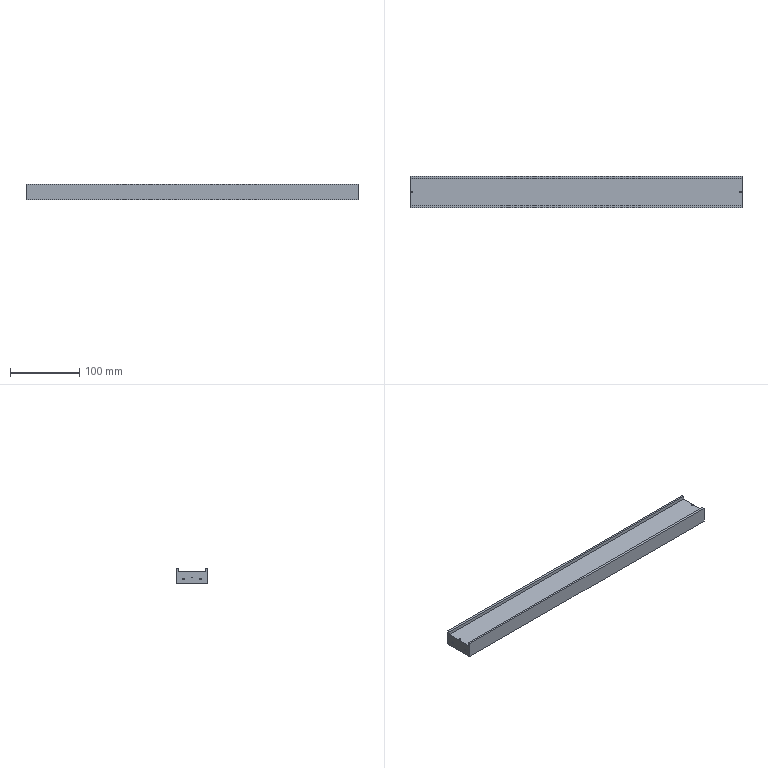Part | NX | 1 solid | 27 faces | box 480 x 45 x 23 mm | volume 314022 mm3 | plane 15 | cone 6 | cylinder 6 | commonest cylinder face diameters 2.5 x6
STEP:
#1=CARTESIAN_POINT('',(240.,-22.5,23.));
#2=VERTEX_POINT('',#1);
#3=CARTESIAN_POINT('',(240.,-19.5,23.));
#4=VERTEX_POINT('',#3);
#5=CARTESIAN_POINT('',(240.,-22.5,23.));
#6=DIRECTION('',(0.,1.,0.));
#7=VECTOR('',#6,1000.);
#8=LINE('',#5,#7);
#9=EDGE_CURVE('',#2,#4,#8,.T.);
#10=ORIENTED_EDGE('',*,*,#9,.T.);
#11=CARTESIAN_POINT('',(-240.,-19.5,23.));
#12=VERTEX_POINT('',#11);
#13=CARTESIAN_POINT('',(-240.,-19.5,23.));
#14=DIRECTION('',(1.,0.,0.));
#15=VECTOR('',#14,1000.);
#16=LINE('',#13,#15);
#17=EDGE_CURVE('',#12,#4,#16,.T.);
#18=ORIENTED_EDGE('',*,*,#17,.F.);
#19=CARTESIAN_POINT('',(-240.,-22.5,23.));
#20=VERTEX_POINT('',#19);
#21=CARTESIAN_POINT('',(-240.,-22.5,23.));
#22=DIRECTION('',(0.,-1.,0.));
#23=VECTOR('',#22,1000.);
#24=LINE('',#21,#23);
#25=EDGE_CURVE('',#12,#20,#24,.T.);
#26=ORIENTED_EDGE('',*,*,#25,.T.);
#27=CARTESIAN_POINT('',(-240.,-22.5,23.));
#28=DIRECTION('',(1.,0.,0.));
#29=VECTOR('',#28,1000.);
#30=LINE('',#27,#29);
#31=EDGE_CURVE('',#20,#2,#30,.T.);
#32=ORIENTED_EDGE('',*,*,#31,.T.);
#33=EDGE_LOOP('',(#10,#18,#26,#32));
#34=FACE_BOUND('',#33,.T.);
#35=CARTESIAN_POINT('',(0.,0.,23.));
#36=DIRECTION('',(0.,0.,-1.));
#37=DIRECTION('',(-1.,0.,0.));
#38=AXIS2_PLACEMENT_3D('',#35,#36,#37);
#39=PLANE('',#38);
#40=ADVANCED_FACE('',(#34),#39,.F.);
#41=CARTESIAN_POINT('',(240.,12.5,5.75));
#42=VERTEX_POINT('',#41);
#43=CARTESIAN_POINT('',(240.,12.5,7.));
#44=DIRECTION('',(1.,0.,0.));
#45=DIRECTION('',(0.,0.,-1.));
#46=AXIS2_PLACEMENT_3D('',#43,#44,#45);
#47=CIRCLE('',#46,1.25);
#48=EDGE_CURVE('',#42,#42,#47,.T.);
#49=ORIENTED_EDGE('',*,*,#48,.F.);
#50=EDGE_LOOP('',(#49));
#51=FACE_BOUND('',#50,.T.);
#52=CARTESIAN_POINT('',(240.,-12.5,5.75));
#53=VERTEX_POINT('',#52);
#54=CARTESIAN_POINT('',(240.,-12.5,7.));
#55=DIRECTION('',(1.,0.,0.));
#56=DIRECTION('',(0.,0.,-1.));
#57=AXIS2_PLACEMENT_3D('',#54,#55,#56);
#58=CIRCLE('',#57,1.25);
#59=EDGE_CURVE('',#53,#53,#58,.T.);
#60=ORIENTED_EDGE('',*,*,#59,.F.);
#61=EDGE_LOOP('',(#60));
#62=FACE_BOUND('',#61,.T.);
#63=CARTESIAN_POINT('',(240.,-19.5,18.));
#64=VERTEX_POINT('',#63);
#65=CARTESIAN_POINT('',(240.,19.5,18.));
#66=VERTEX_POINT('',#65);
#67=CARTESIAN_POINT('',(240.,-19.5,18.));
#68=DIRECTION('',(0.,1.,0.));
#69=VECTOR('',#68,1000.);
#70=LINE('',#67,#69);
#71=EDGE_CURVE('',#64,#66,#70,.T.);
#72=ORIENTED_EDGE('',*,*,#71,.F.);
#73=CARTESIAN_POINT('',(240.,-19.5,18.));
#74=DIRECTION('',(0.,0.,1.));
#75=VECTOR('',#74,1000.);
#76=LINE('',#73,#75);
#77=EDGE_CURVE('',#64,#4,#76,.T.);
#78=ORIENTED_EDGE('',*,*,#77,.T.);
#79=ORIENTED_EDGE('',*,*,#9,.F.);
#80=CARTESIAN_POINT('',(240.,-22.5,0.));
#81=VERTEX_POINT('',#80);
#82=CARTESIAN_POINT('',(240.,-22.5,23.));
#83=DIRECTION('',(0.,0.,-1.));
#84=VECTOR('',#83,1000.);
#85=LINE('',#82,#84);
#86=EDGE_CURVE('',#2,#81,#85,.T.);
#87=ORIENTED_EDGE('',*,*,#86,.T.);
#88=CARTESIAN_POINT('',(240.,22.5,0.));
#89=VERTEX_POINT('',#88);
#90=CARTESIAN_POINT('',(240.,-22.5,0.));
#91=DIRECTION('',(0.,1.,0.));
#92=VECTOR('',#91,1000.);
#93=LINE('',#90,#92);
#94=EDGE_CURVE('',#81,#89,#93,.T.);
#95=ORIENTED_EDGE('',*,*,#94,.T.);
#96=CARTESIAN_POINT('',(240.,22.5,23.));
#97=VERTEX_POINT('',#96);
#98=CARTESIAN_POINT('',(240.,22.5,23.));
#99=DIRECTION('',(0.,0.,-1.));
#100=VECTOR('',#99,1000.);
#101=LINE('',#98,#100);
#102=EDGE_CURVE('',#97,#89,#101,.T.);
#103=ORIENTED_EDGE('',*,*,#102,.F.);
#104=CARTESIAN_POINT('',(240.,19.5,23.));
#105=VERTEX_POINT('',#104);
#106=CARTESIAN_POINT('',(240.,-22.5,23.));
#107=DIRECTION('',(0.,1.,0.));
#108=VECTOR('',#107,1000.);
#109=LINE('',#106,#108);
#110=EDGE_CURVE('',#105,#97,#109,.T.);
#111=ORIENTED_EDGE('',*,*,#110,.F.);
#112=CARTESIAN_POINT('',(240.,19.5,18.));
#113=DIRECTION('',(0.,0.,1.));
#114=VECTOR('',#113,1000.);
#115=LINE('',#112,#114);
#116=EDGE_CURVE('',#66,#105,#115,.T.);
#117=ORIENTED_EDGE('',*,*,#116,.F.);
#118=EDGE_LOOP('',(#72,#78,#79,#87,#95,#103,#111,#117));
#119=FACE_BOUND('',#118,.T.);
#120=CARTESIAN_POINT('',(240.,-22.5,23.));
#121=DIRECTION('',(-1.,0.,0.));
#122=DIRECTION('',(0.,0.,1.));
#123=AXIS2_PLACEMENT_3D('',#120,#121,#122);
#124=PLANE('',#123);
#125=ADVANCED_FACE('',(#51,#62,#119),#124,.F.);
#126=CARTESIAN_POINT('',(-240.,22.5,0.));
#127=VERTEX_POINT('',#126);
#128=CARTESIAN_POINT('',(-240.,22.5,0.));
#129=DIRECTION('',(-1.,0.,0.));
#130=VECTOR('',#129,1000.);
#131=LINE('',#128,#130);
#132=EDGE_CURVE('',#89,#127,#131,.T.);
#133=ORIENTED_EDGE('',*,*,#132,.T.);
#134=CARTESIAN_POINT('',(-240.,22.5,23.));
#135=VERTEX_POINT('',#134);
#136=CARTESIAN_POINT('',(-240.,22.5,23.));
#137=DIRECTION('',(0.,0.,-1.));
#138=VECTOR('',#137,1000.);
#139=LINE('',#136,#138);
#140=EDGE_CURVE('',#135,#127,#139,.T.);
#141=ORIENTED_EDGE('',*,*,#140,.F.);
#142=CARTESIAN_POINT('',(-240.,22.5,23.));
#143=DIRECTION('',(-1.,0.,0.));
#144=VECTOR('',#143,1000.);
#145=LINE('',#142,#144);
#146=EDGE_CURVE('',#97,#135,#145,.T.);
#147=ORIENTED_EDGE('',*,*,#146,.F.);
#148=ORIENTED_EDGE('',*,*,#102,.T.);
#149=EDGE_LOOP('',(#133,#141,#147,#148));
#150=FACE_BOUND('',#149,.T.);
#151=CARTESIAN_POINT('',(-240.,22.5,23.));
#152=DIRECTION('',(0.,-1.,0.));
#153=DIRECTION('',(0.,0.,-1.));
#154=AXIS2_PLACEMENT_3D('',#151,#152,#153);
#155=PLANE('',#154);
#156=ADVANCED_FACE('',(#150),#155,.F.);
#157=CARTESIAN_POINT('',(-240.,12.5,8.25));
#158=VERTEX_POINT('',#157);
#159=CARTESIAN_POINT('',(-240.,12.5,7.));
#160=DIRECTION('',(-1.,0.,0.));
#161=DIRECTION('',(0.,0.,1.));
#162=AXIS2_PLACEMENT_3D('',#159,#160,#161);
#163=CIRCLE('',#162,1.25);
#164=EDGE_CURVE('',#158,#158,#163,.T.);
#165=ORIENTED_EDGE('',*,*,#164,.F.);
#166=EDGE_LOOP('',(#165));
#167=FACE_BOUND('',#166,.T.);
#168=CARTESIAN_POINT('',(-240.,-12.5,8.25));
#169=VERTEX_POINT('',#168);
#170=CARTESIAN_POINT('',(-240.,-12.5,7.));
#171=DIRECTION('',(-1.,0.,0.));
#172=DIRECTION('',(0.,0.,1.));
#173=AXIS2_PLACEMENT_3D('',#170,#171,#172);
#174=CIRCLE('',#173,1.25);
#175=EDGE_CURVE('',#169,#169,#174,.T.);
#176=ORIENTED_EDGE('',*,*,#175,.F.);
#177=EDGE_LOOP('',(#176));
#178=FACE_BOUND('',#177,.T.);
#179=ORIENTED_EDGE('',*,*,#25,.F.);
#180=CARTESIAN_POINT('',(-240.,-19.5,18.));
#181=VERTEX_POINT('',#180);
#182=CARTESIAN_POINT('',(-240.,-19.5,18.));
#183=DIRECTION('',(0.,0.,1.));
#184=VECTOR('',#183,1000.);
#185=LINE('',#182,#184);
#186=EDGE_CURVE('',#181,#12,#185,.T.);
#187=ORIENTED_EDGE('',*,*,#186,.F.);
#188=CARTESIAN_POINT('',(-240.,19.5,18.));
#189=VERTEX_POINT('',#188);
#190=CARTESIAN_POINT('',(-240.,-19.5,18.));
#191=DIRECTION('',(0.,-1.,0.));
#192=VECTOR('',#191,1000.);
#193=LINE('',#190,#192);
#194=EDGE_CURVE('',#189,#181,#193,.T.);
#195=ORIENTED_EDGE('',*,*,#194,.F.);
#196=CARTESIAN_POINT('',(-240.,19.5,23.));
#197=VERTEX_POINT('',#196);
#198=CARTESIAN_POINT('',(-240.,19.5,18.));
#199=DIRECTION('',(0.,0.,1.));
#200=VECTOR('',#199,1000.);
#201=LINE('',#198,#200);
#202=EDGE_CURVE('',#189,#197,#201,.T.);
#203=ORIENTED_EDGE('',*,*,#202,.T.);
#204=CARTESIAN_POINT('',(-240.,-22.5,23.));
#205=DIRECTION('',(0.,-1.,0.));
#206=VECTOR('',#205,1000.);
#207=LINE('',#204,#206);
#208=EDGE_CURVE('',#135,#197,#207,.T.);
#209=ORIENTED_EDGE('',*,*,#208,.F.);
#210=ORIENTED_EDGE('',*,*,#140,.T.);
#211=CARTESIAN_POINT('',(-240.,-22.5,0.));
#212=VERTEX_POINT('',#211);
#213=CARTESIAN_POINT('',(-240.,-22.5,0.));
#214=DIRECTION('',(0.,-1.,0.));
#215=VECTOR('',#214,1000.);
#216=LINE('',#213,#215);
#217=EDGE_CURVE('',#127,#212,#216,.T.);
#218=ORIENTED_EDGE('',*,*,#217,.T.);
#219=CARTESIAN_POINT('',(-240.,-22.5,23.));
#220=DIRECTION('',(0.,0.,-1.));
#221=VECTOR('',#220,1000.);
#222=LINE('',#219,#221);
#223=EDGE_CURVE('',#20,#212,#222,.T.);
#224=ORIENTED_EDGE('',*,*,#223,.F.);
#225=EDGE_LOOP('',(#179,#187,#195,#203,#209,#210,#218,#224));
#226=FACE_BOUND('',#225,.T.);
#227=CARTESIAN_POINT('',(-240.,-22.5,23.));
#228=DIRECTION('',(1.,0.,0.));
#229=DIRECTION('',(0.,0.,-1.));
#230=AXIS2_PLACEMENT_3D('',#227,#228,#229);
#231=PLANE('',#230);
#232=ADVANCED_FACE('',(#167,#178,#226),#231,.F.);
#233=CARTESIAN_POINT('',(-240.,-22.5,0.));
#234=DIRECTION('',(1.,0.,0.));
#235=VECTOR('',#234,1000.);
#236=LINE('',#233,#235);
#237=EDGE_CURVE('',#212,#81,#236,.T.);
#238=ORIENTED_EDGE('',*,*,#237,.T.);
#239=ORIENTED_EDGE('',*,*,#86,.F.);
#240=ORIENTED_EDGE('',*,*,#31,.F.);
#241=ORIENTED_EDGE('',*,*,#223,.T.);
#242=EDGE_LOOP('',(#238,#239,#240,#241));
#243=FACE_BOUND('',#242,.T.);
#244=CARTESIAN_POINT('',(-240.,-22.5,23.));
#245=DIRECTION('',(0.,1.,0.));
#246=DIRECTION('',(0.,0.,1.));
#247=AXIS2_PLACEMENT_3D('',#244,#245,#246);
#248=PLANE('',#247);
#249=ADVANCED_FACE('',(#243),#248,.F.);
#250=ORIENTED_EDGE('',*,*,#208,.T.);
#251=CARTESIAN_POINT('',(-240.,19.5,23.));
#252=DIRECTION('',(-1.,0.,0.));
#253=VECTOR('',#252,1000.);
#254=LINE('',#251,#253);
#255=EDGE_CURVE('',#105,#197,#254,.T.);
#256=ORIENTED_EDGE('',*,*,#255,.F.);
#257=ORIENTED_EDGE('',*,*,#110,.T.);
#258=ORIENTED_EDGE('',*,*,#146,.T.);
#259=EDGE_LOOP('',(#250,#256,#257,#258));
#260=FACE_BOUND('',#259,.T.);
#261=CARTESIAN_POINT('',(0.,0.,23.));
#262=DIRECTION('',(0.,0.,-1.));
#263=DIRECTION('',(-1.,0.,0.));
#264=AXIS2_PLACEMENT_3D('',#261,#262,#263);
#265=PLANE('',#264);
#266=ADVANCED_FACE('',(#260),#265,.F.);
#267=CARTESIAN_POINT('',(-234.,-19.,0.));
#268=VERTEX_POINT('',#267);
#269=CARTESIAN_POINT('',(-234.,19.,0.));
#270=VERTEX_POINT('',#269);
#271=CARTESIAN_POINT('',(-234.,-19.,0.));
#272=DIRECTION('',(0.,1.,0.));
#273=VECTOR('',#272,1000.);
#274=LINE('',#271,#273);
#275=EDGE_CURVE('',#268,#270,#274,.T.);
#276=ORIENTED_EDGE('',*,*,#275,.F.);
#277=CARTESIAN_POINT('',(234.,-19.,0.));
#278=VERTEX_POINT('',#277);
#279=CARTESIAN_POINT('',(234.,-19.,0.));
#280=DIRECTION('',(-1.,0.,0.));
#281=VECTOR('',#280,1000.);
#282=LINE('',#279,#281);
#283=EDGE_CURVE('',#278,#268,#282,.T.);
#284=ORIENTED_EDGE('',*,*,#283,.F.);
#285=CARTESIAN_POINT('',(234.,19.,0.));
#286=VERTEX_POINT('',#285);
#287=CARTESIAN_POINT('',(234.,-19.,0.));
#288=DIRECTION('',(0.,-1.,0.));
#289=VECTOR('',#288,1000.);
#290=LINE('',#287,#289);
#291=EDGE_CURVE('',#286,#278,#290,.T.);
#292=ORIENTED_EDGE('',*,*,#291,.F.);
#293=CARTESIAN_POINT('',(234.,19.,0.));
#294=DIRECTION('',(1.,0.,0.));
#295=VECTOR('',#294,1000.);
#296=LINE('',#293,#295);
#297=EDGE_CURVE('',#270,#286,#296,.T.);
#298=ORIENTED_EDGE('',*,*,#297,.F.);
#299=EDGE_LOOP('',(#276,#284,#292,#298));
#300=FACE_BOUND('',#299,.T.);
#301=ORIENTED_EDGE('',*,*,#94,.F.);
#302=ORIENTED_EDGE('',*,*,#237,.F.);
#303=ORIENTED_EDGE('',*,*,#217,.F.);
#304=ORIENTED_EDGE('',*,*,#132,.F.);
#305=EDGE_LOOP('',(#301,#302,#303,#304));
#306=FACE_BOUND('',#305,.T.);
#307=CARTESIAN_POINT('',(0.,0.,0.));
#308=DIRECTION('',(0.,0.,-1.));
#309=DIRECTION('',(-1.,0.,0.));
#310=AXIS2_PLACEMENT_3D('',#307,#308,#309);
#311=PLANE('',#310);
#312=ADVANCED_FACE('',(#300,#306),#311,.T.);
#313=ORIENTED_EDGE('',*,*,#17,.T.);
#314=ORIENTED_EDGE('',*,*,#77,.F.);
#315=CARTESIAN_POINT('',(-240.,-19.5,18.));
#316=DIRECTION('',(1.,0.,0.));
#317=VECTOR('',#316,1000.);
#318=LINE('',#315,#317);
#319=EDGE_CURVE('',#181,#64,#318,.T.);
#320=ORIENTED_EDGE('',*,*,#319,.F.);
#321=ORIENTED_EDGE('',*,*,#186,.T.);
#322=EDGE_LOOP('',(#313,#314,#320,#321));
#323=FACE_BOUND('',#322,.T.);
#324=CARTESIAN_POINT('',(-240.,-19.5,18.));
#325=DIRECTION('',(0.,-1.,0.));
#326=DIRECTION('',(0.,0.,-1.));
#327=AXIS2_PLACEMENT_3D('',#324,#325,#326);
#328=PLANE('',#327);
#329=ADVANCED_FACE('',(#323),#328,.F.);
#330=ORIENTED_EDGE('',*,*,#255,.T.);
#331=ORIENTED_EDGE('',*,*,#202,.F.);
#332=CARTESIAN_POINT('',(-240.,19.5,18.));
#333=DIRECTION('',(-1.,0.,0.));
#334=VECTOR('',#333,1000.);
#335=LINE('',#332,#334);
#336=EDGE_CURVE('',#66,#189,#335,.T.);
#337=ORIENTED_EDGE('',*,*,#336,.F.);
#338=ORIENTED_EDGE('',*,*,#116,.T.);
#339=EDGE_LOOP('',(#330,#331,#337,#338));
#340=FACE_BOUND('',#339,.T.);
#341=CARTESIAN_POINT('',(-240.,19.5,18.));
#342=DIRECTION('',(0.,1.,0.));
#343=DIRECTION('',(0.,0.,1.));
#344=AXIS2_PLACEMENT_3D('',#341,#342,#343);
#345=PLANE('',#344);
#346=ADVANCED_FACE('',(#340),#345,.F.);
#347=CARTESIAN_POINT('',(-236.25,0.,18.));
#348=VERTEX_POINT('',#347);
#349=CARTESIAN_POINT('',(-237.5,0.,18.));
#350=DIRECTION('',(0.,0.,1.));
#351=DIRECTION('',(1.,0.,0.));
#352=AXIS2_PLACEMENT_3D('',#349,#350,#351);
#353=CIRCLE('',#352,1.25);
#354=EDGE_CURVE('',#348,#348,#353,.T.);
#355=ORIENTED_EDGE('',*,*,#354,.F.);
#356=EDGE_LOOP('',(#355));
#357=FACE_BOUND('',#356,.T.);
#358=CARTESIAN_POINT('',(238.75,0.,18.));
#359=VERTEX_POINT('',#358);
#360=CARTESIAN_POINT('',(237.5,0.,18.));
#361=DIRECTION('',(0.,0.,1.));
#362=DIRECTION('',(1.,0.,0.));
#363=AXIS2_PLACEMENT_3D('',#360,#361,#362);
#364=CIRCLE('',#363,1.25);
#365=EDGE_CURVE('',#359,#359,#364,.T.);
#366=ORIENTED_EDGE('',*,*,#365,.F.);
#367=EDGE_LOOP('',(#366));
#368=FACE_BOUND('',#367,.T.);
#369=ORIENTED_EDGE('',*,*,#71,.T.);
#370=ORIENTED_EDGE('',*,*,#336,.T.);
#371=ORIENTED_EDGE('',*,*,#194,.T.);
#372=ORIENTED_EDGE('',*,*,#319,.T.);
#373=EDGE_LOOP('',(#369,#370,#371,#372));
#374=FACE_BOUND('',#373,.T.);
#375=CARTESIAN_POINT('',(0.,0.,18.));
#376=DIRECTION('',(0.,0.,-1.));
#377=DIRECTION('',(-1.,0.,0.));
#378=AXIS2_PLACEMENT_3D('',#375,#376,#377);
#379=PLANE('',#378);
#380=ADVANCED_FACE('',(#357,#368,#374),#379,.F.);
#381=CARTESIAN_POINT('',(237.5,0.,8.749));
#382=VERTEX_POINT('',#381);
#383=VERTEX_LOOP('',#382);
#384=FACE_BOUND('',#383,.T.);
#385=CARTESIAN_POINT('',(238.75,0.,9.5));
#386=VERTEX_POINT('',#385);
#387=CARTESIAN_POINT('',(237.5,0.,9.5));
#388=DIRECTION('',(0.,0.,1.));
#389=DIRECTION('',(1.,0.,0.));
#390=AXIS2_PLACEMENT_3D('',#387,#388,#389);
#391=CIRCLE('',#390,1.25);
#392=EDGE_CURVE('',#386,#386,#391,.T.);
#393=ORIENTED_EDGE('',*,*,#392,.T.);
#394=EDGE_LOOP('',(#393));
#395=FACE_BOUND('',#394,.T.);
#396=CARTESIAN_POINT('',(237.5,0.,9.5));
#397=DIRECTION('',(0.,0.,1.));
#398=DIRECTION('',(1.,0.,0.));
#399=AXIS2_PLACEMENT_3D('',#396,#397,#398);
#400=CONICAL_SURFACE('',#399,1.25,1.03);
#401=ADVANCED_FACE('',(#384,#395),#400,.F.);
#402=ORIENTED_EDGE('',*,*,#392,.F.);
#403=EDGE_LOOP('',(#402));
#404=FACE_BOUND('',#403,.T.);
#405=ORIENTED_EDGE('',*,*,#365,.T.);
#406=EDGE_LOOP('',(#405));
#407=FACE_BOUND('',#406,.T.);
#408=CARTESIAN_POINT('',(237.5,0.,18.));
#409=DIRECTION('',(0.,0.,1.));
#410=DIRECTION('',(1.,0.,0.));
#411=AXIS2_PLACEMENT_3D('',#408,#409,#410);
#412=CYLINDRICAL_SURFACE('',#411,1.25);
#413=ADVANCED_FACE('',(#404,#407),#412,.F.);
#414=CARTESIAN_POINT('',(-237.5,0.,8.749));
#415=VERTEX_POINT('',#414);
#416=VERTEX_LOOP('',#415);
#417=FACE_BOUND('',#416,.T.);
#418=CARTESIAN_POINT('',(-236.25,0.,9.5));
#419=VERTEX_POINT('',#418);
#420=CARTESIAN_POINT('',(-237.5,0.,9.5));
#421=DIRECTION('',(0.,0.,1.));
#422=DIRECTION('',(1.,0.,0.));
#423=AXIS2_PLACEMENT_3D('',#420,#421,#422);
#424=CIRCLE('',#423,1.25);
#425=EDGE_CURVE('',#419,#419,#424,.T.);
#426=ORIENTED_EDGE('',*,*,#425,.T.);
#427=EDGE_LOOP('',(#426));
#428=FACE_BOUND('',#427,.T.);
#429=CARTESIAN_POINT('',(-237.5,0.,9.5));
#430=DIRECTION('',(0.,0.,1.));
#431=DIRECTION('',(1.,0.,0.));
#432=AXIS2_PLACEMENT_3D('',#429,#430,#431);
#433=CONICAL_SURFACE('',#432,1.25,1.03);
#434=ADVANCED_FACE('',(#417,#428),#433,.F.);
#435=ORIENTED_EDGE('',*,*,#425,.F.);
#436=EDGE_LOOP('',(#435));
#437=FACE_BOUND('',#436,.T.);
#438=ORIENTED_EDGE('',*,*,#354,.T.);
#439=EDGE_LOOP('',(#438));
#440=FACE_BOUND('',#439,.T.);
#441=CARTESIAN_POINT('',(-237.5,0.,18.));
#442=DIRECTION('',(0.,0.,1.));
#443=DIRECTION('',(1.,0.,0.));
#444=AXIS2_PLACEMENT_3D('',#441,#442,#443);
#445=CYLINDRICAL_SURFACE('',#444,1.25);
#446=ADVANCED_FACE('',(#437,#440),#445,.F.);
#447=CARTESIAN_POINT('',(-230.749,-12.5,7.));
#448=VERTEX_POINT('',#447);
#449=VERTEX_LOOP('',#448);
#450=FACE_BOUND('',#449,.T.);
#451=CARTESIAN_POINT('',(-231.5,-12.5,8.25));
#452=VERTEX_POINT('',#451);
#453=CARTESIAN_POINT('',(-231.5,-12.5,7.));
#454=DIRECTION('',(-1.,0.,0.));
#455=DIRECTION('',(0.,0.,1.));
#456=AXIS2_PLACEMENT_3D('',#453,#454,#455);
#457=CIRCLE('',#456,1.25);
#458=EDGE_CURVE('',#452,#452,#457,.T.);
#459=ORIENTED_EDGE('',*,*,#458,.T.);
#460=EDGE_LOOP('',(#459));
#461=FACE_BOUND('',#460,.T.);
#462=CARTESIAN_POINT('',(-231.5,-12.5,7.));
#463=DIRECTION('',(-1.,0.,0.));
#464=DIRECTION('',(0.,0.,1.));
#465=AXIS2_PLACEMENT_3D('',#462,#463,#464);
#466=CONICAL_SURFACE('',#465,1.25,1.03);
#467=ADVANCED_FACE('',(#450,#461),#466,.F.);
#468=ORIENTED_EDGE('',*,*,#458,.F.);
#469=EDGE_LOOP('',(#468));
#470=FACE_BOUND('',#469,.T.);
#471=ORIENTED_EDGE('',*,*,#175,.T.);
#472=EDGE_LOOP('',(#471));
#473=FACE_BOUND('',#472,.T.);
#474=CARTESIAN_POINT('',(-240.,-12.5,7.));
#475=DIRECTION('',(-1.,0.,0.));
#476=DIRECTION('',(0.,0.,1.));
#477=AXIS2_PLACEMENT_3D('',#474,#475,#476);
#478=CYLINDRICAL_SURFACE('',#477,1.25);
#479=ADVANCED_FACE('',(#470,#473),#478,.F.);
#480=CARTESIAN_POINT('',(-230.749,12.5,7.));
#481=VERTEX_POINT('',#480);
#482=VERTEX_LOOP('',#481);
#483=FACE_BOUND('',#482,.T.);
#484=CARTESIAN_POINT('',(-231.5,12.5,8.25));
#485=VERTEX_POINT('',#484);
#486=CARTESIAN_POINT('',(-231.5,12.5,7.));
#487=DIRECTION('',(-1.,0.,0.));
#488=DIRECTION('',(0.,0.,1.));
#489=AXIS2_PLACEMENT_3D('',#486,#487,#488);
#490=CIRCLE('',#489,1.25);
#491=EDGE_CURVE('',#485,#485,#490,.T.);
#492=ORIENTED_EDGE('',*,*,#491,.T.);
#493=EDGE_LOOP('',(#492));
#494=FACE_BOUND('',#493,.T.);
#495=CARTESIAN_POINT('',(-231.5,12.5,7.));
#496=DIRECTION('',(-1.,0.,0.));
#497=DIRECTION('',(0.,0.,1.));
#498=AXIS2_PLACEMENT_3D('',#495,#496,#497);
#499=CONICAL_SURFACE('',#498,1.25,1.03);
#500=ADVANCED_FACE('',(#483,#494),#499,.F.);
#501=ORIENTED_EDGE('',*,*,#491,.F.);
#502=EDGE_LOOP('',(#501));
#503=FACE_BOUND('',#502,.T.);
#504=ORIENTED_EDGE('',*,*,#164,.T.);
#505=EDGE_LOOP('',(#504));
#506=FACE_BOUND('',#505,.T.);
#507=CARTESIAN_POINT('',(-240.,12.5,7.));
#508=DIRECTION('',(-1.,0.,0.));
#509=DIRECTION('',(0.,0.,1.));
#510=AXIS2_PLACEMENT_3D('',#507,#508,#509);
#511=CYLINDRICAL_SURFACE('',#510,1.25);
#512=ADVANCED_FACE('',(#503,#506),#511,.F.);
#513=CARTESIAN_POINT('',(230.749,-12.5,7.));
#514=VERTEX_POINT('',#513);
#515=VERTEX_LOOP('',#514);
#516=FACE_BOUND('',#515,.T.);
#517=CARTESIAN_POINT('',(231.5,-12.5,5.75));
#518=VERTEX_POINT('',#517);
#519=CARTESIAN_POINT('',(231.5,-12.5,7.));
#520=DIRECTION('',(1.,0.,0.));
#521=DIRECTION('',(0.,0.,-1.));
#522=AXIS2_PLACEMENT_3D('',#519,#520,#521);
#523=CIRCLE('',#522,1.25);
#524=EDGE_CURVE('',#518,#518,#523,.T.);
#525=ORIENTED_EDGE('',*,*,#524,.T.);
#526=EDGE_LOOP('',(#525));
#527=FACE_BOUND('',#526,.T.);
#528=CARTESIAN_POINT('',(231.5,-12.5,7.));
#529=DIRECTION('',(1.,0.,0.));
#530=DIRECTION('',(0.,0.,-1.));
#531=AXIS2_PLACEMENT_3D('',#528,#529,#530);
#532=CONICAL_SURFACE('',#531,1.25,1.03);
#533=ADVANCED_FACE('',(#516,#527),#532,.F.);
#534=ORIENTED_EDGE('',*,*,#524,.F.);
#535=EDGE_LOOP('',(#534));
#536=FACE_BOUND('',#535,.T.);
#537=ORIENTED_EDGE('',*,*,#59,.T.);
#538=EDGE_LOOP('',(#537));
#539=FACE_BOUND('',#538,.T.);
#540=CARTESIAN_POINT('',(240.,-12.5,7.));
#541=DIRECTION('',(1.,0.,0.));
#542=DIRECTION('',(0.,0.,-1.));
#543=AXIS2_PLACEMENT_3D('',#540,#541,#542);
#544=CYLINDRICAL_SURFACE('',#543,1.25);
#545=ADVANCED_FACE('',(#536,#539),#544,.F.);
#546=CARTESIAN_POINT('',(230.749,12.5,7.));
#547=VERTEX_POINT('',#546);
#548=VERTEX_LOOP('',#547);
#549=FACE_BOUND('',#548,.T.);
#550=CARTESIAN_POINT('',(231.5,12.5,5.75));
#551=VERTEX_POINT('',#550);
#552=CARTESIAN_POINT('',(231.5,12.5,7.));
#553=DIRECTION('',(1.,0.,0.));
#554=DIRECTION('',(0.,0.,-1.));
#555=AXIS2_PLACEMENT_3D('',#552,#553,#554);
#556=CIRCLE('',#555,1.25);
#557=EDGE_CURVE('',#551,#551,#556,.T.);
#558=ORIENTED_EDGE('',*,*,#557,.T.);
#559=EDGE_LOOP('',(#558));
#560=FACE_BOUND('',#559,.T.);
#561=CARTESIAN_POINT('',(231.5,12.5,7.));
#562=DIRECTION('',(1.,0.,0.));
#563=DIRECTION('',(0.,0.,-1.));
#564=AXIS2_PLACEMENT_3D('',#561,#562,#563);
#565=CONICAL_SURFACE('',#564,1.25,1.03);
#566=ADVANCED_FACE('',(#549,#560),#565,.F.);
#567=ORIENTED_EDGE('',*,*,#557,.F.);
#568=EDGE_LOOP('',(#567));
#569=FACE_BOUND('',#568,.T.);
#570=ORIENTED_EDGE('',*,*,#48,.T.);
#571=EDGE_LOOP('',(#570));
#572=FACE_BOUND('',#571,.T.);
#573=CARTESIAN_POINT('',(240.,12.5,7.));
#574=DIRECTION('',(1.,0.,0.));
#575=DIRECTION('',(0.,0.,-1.));
#576=AXIS2_PLACEMENT_3D('',#573,#574,#575);
#577=CYLINDRICAL_SURFACE('',#576,1.25);
#578=ADVANCED_FACE('',(#569,#572),#577,.F.);
#579=ORIENTED_EDGE('',*,*,#275,.T.);
#580=CARTESIAN_POINT('',(-234.,19.,5.));
#581=VERTEX_POINT('',#580);
#582=CARTESIAN_POINT('',(-234.,19.,5.));
#583=DIRECTION('',(0.,0.,-1.));
#584=VECTOR('',#583,1000.);
#585=LINE('',#582,#584);
#586=EDGE_CURVE('',#581,#270,#585,.T.);
#587=ORIENTED_EDGE('',*,*,#586,.F.);
#588=CARTESIAN_POINT('',(-234.,-19.,5.));
#589=VERTEX_POINT('',#588);
#590=CARTESIAN_POINT('',(-234.,-19.,5.));
#591=DIRECTION('',(0.,1.,0.));
#592=VECTOR('',#591,1000.);
#593=LINE('',#590,#592);
#594=EDGE_CURVE('',#589,#581,#593,.T.);
#595=ORIENTED_EDGE('',*,*,#594,.F.);
#596=CARTESIAN_POINT('',(-234.,-19.,5.));
#597=DIRECTION('',(0.,0.,-1.));
#598=VECTOR('',#597,1000.);
#599=LINE('',#596,#598);
#600=EDGE_CURVE('',#589,#268,#599,.T.);
#601=ORIENTED_EDGE('',*,*,#600,.T.);
#602=EDGE_LOOP('',(#579,#587,#595,#601));
#603=FACE_BOUND('',#602,.T.);
#604=CARTESIAN_POINT('',(-234.,-19.,5.));
#605=DIRECTION('',(-1.,0.,0.));
#606=DIRECTION('',(0.,0.,1.));
#607=AXIS2_PLACEMENT_3D('',#604,#605,#606);
#608=PLANE('',#607);
#609=ADVANCED_FACE('',(#603),#608,.F.);
#610=ORIENTED_EDGE('',*,*,#283,.T.);
#611=ORIENTED_EDGE('',*,*,#600,.F.);
#612=CARTESIAN_POINT('',(234.,-19.,5.));
#613=VERTEX_POINT('',#612);
#614=CARTESIAN_POINT('',(234.,-19.,5.));
#615=DIRECTION('',(-1.,0.,0.));
#616=VECTOR('',#615,1000.);
#617=LINE('',#614,#616);
#618=EDGE_CURVE('',#613,#589,#617,.T.);
#619=ORIENTED_EDGE('',*,*,#618,.F.);
#620=CARTESIAN_POINT('',(234.,-19.,5.));
#621=DIRECTION('',(0.,0.,-1.));
#622=VECTOR('',#621,1000.);
#623=LINE('',#620,#622);
#624=EDGE_CURVE('',#613,#278,#623,.T.);
#625=ORIENTED_EDGE('',*,*,#624,.T.);
#626=EDGE_LOOP('',(#610,#611,#619,#625));
#627=FACE_BOUND('',#626,.T.);
#628=CARTESIAN_POINT('',(234.,-19.,5.));
#629=DIRECTION('',(0.,-1.,0.));
#630=DIRECTION('',(0.,0.,-1.));
#631=AXIS2_PLACEMENT_3D('',#628,#629,#630);
#632=PLANE('',#631);
#633=ADVANCED_FACE('',(#627),#632,.F.);
#634=ORIENTED_EDGE('',*,*,#291,.T.);
#635=ORIENTED_EDGE('',*,*,#624,.F.);
#636=CARTESIAN_POINT('',(234.,19.,5.));
#637=VERTEX_POINT('',#636);
#638=CARTESIAN_POINT('',(234.,-19.,5.));
#639=DIRECTION('',(0.,-1.,0.));
#640=VECTOR('',#639,1000.);
#641=LINE('',#638,#640);
#642=EDGE_CURVE('',#637,#613,#641,.T.);
#643=ORIENTED_EDGE('',*,*,#642,.F.);
#644=CARTESIAN_POINT('',(234.,19.,5.));
#645=DIRECTION('',(0.,0.,-1.));
#646=VECTOR('',#645,1000.);
#647=LINE('',#644,#646);
#648=EDGE_CURVE('',#637,#286,#647,.T.);
#649=ORIENTED_EDGE('',*,*,#648,.T.);
#650=EDGE_LOOP('',(#634,#635,#643,#649));
#651=FACE_BOUND('',#650,.T.);
#652=CARTESIAN_POINT('',(234.,-19.,5.));
#653=DIRECTION('',(1.,0.,0.));
#654=DIRECTION('',(0.,0.,-1.));
#655=AXIS2_PLACEMENT_3D('',#652,#653,#654);
#656=PLANE('',#655);
#657=ADVANCED_FACE('',(#651),#656,.F.);
#658=ORIENTED_EDGE('',*,*,#297,.T.);
#659=ORIENTED_EDGE('',*,*,#648,.F.);
#660=CARTESIAN_POINT('',(234.,19.,5.));
#661=DIRECTION('',(1.,0.,0.));
#662=VECTOR('',#661,1000.);
#663=LINE('',#660,#662);
#664=EDGE_CURVE('',#581,#637,#663,.T.);
#665=ORIENTED_EDGE('',*,*,#664,.F.);
#666=ORIENTED_EDGE('',*,*,#586,.T.);
#667=EDGE_LOOP('',(#658,#659,#665,#666));
#668=FACE_BOUND('',#667,.T.);
#669=CARTESIAN_POINT('',(234.,19.,5.));
#670=DIRECTION('',(0.,1.,0.));
#671=DIRECTION('',(0.,0.,1.));
#672=AXIS2_PLACEMENT_3D('',#669,#670,#671);
#673=PLANE('',#672);
#674=ADVANCED_FACE('',(#668),#673,.F.);
#675=ORIENTED_EDGE('',*,*,#594,.T.);
#676=ORIENTED_EDGE('',*,*,#664,.T.);
#677=ORIENTED_EDGE('',*,*,#642,.T.);
#678=ORIENTED_EDGE('',*,*,#618,.T.);
#679=EDGE_LOOP('',(#675,#676,#677,#678));
#680=FACE_BOUND('',#679,.T.);
#681=CARTESIAN_POINT('',(0.,0.,5.));
#682=DIRECTION('',(0.,0.,1.));
#683=DIRECTION('',(1.,0.,0.));
#684=AXIS2_PLACEMENT_3D('',#681,#682,#683);
#685=PLANE('',#684);
#686=ADVANCED_FACE('',(#680),#685,.F.);
#687=CLOSED_SHELL('',(#40,#125,#156,#232,#249,#266,#312,#329,#346,#380,#401,#413,#434,#446,#467,#479,#500,#512,#533,#545,#566,#578,#609,#633,#657,#674,#686));
#688=MANIFOLD_SOLID_BREP('',#687);
#689=(LENGTH_UNIT()NAMED_UNIT(*)SI_UNIT(.MILLI.,.METRE.));
#690=UNCERTAINTY_MEASURE_WITH_UNIT(LENGTH_MEASURE(0.00001),#689,'','');
#691=(NAMED_UNIT(*)PLANE_ANGLE_UNIT()SI_UNIT($,.RADIAN.));
#692=(NAMED_UNIT(*)SI_UNIT($,.STERADIAN.)SOLID_ANGLE_UNIT());
#693=(GEOMETRIC_REPRESENTATION_CONTEXT(3)GLOBAL_UNCERTAINTY_ASSIGNED_CONTEXT((#690))GLOBAL_UNIT_ASSIGNED_CONTEXT((#689,#691,#692))REPRESENTATION_CONTEXT('',''));
#694=ADVANCED_BREP_SHAPE_REPRESENTATION('',(#688),#693);